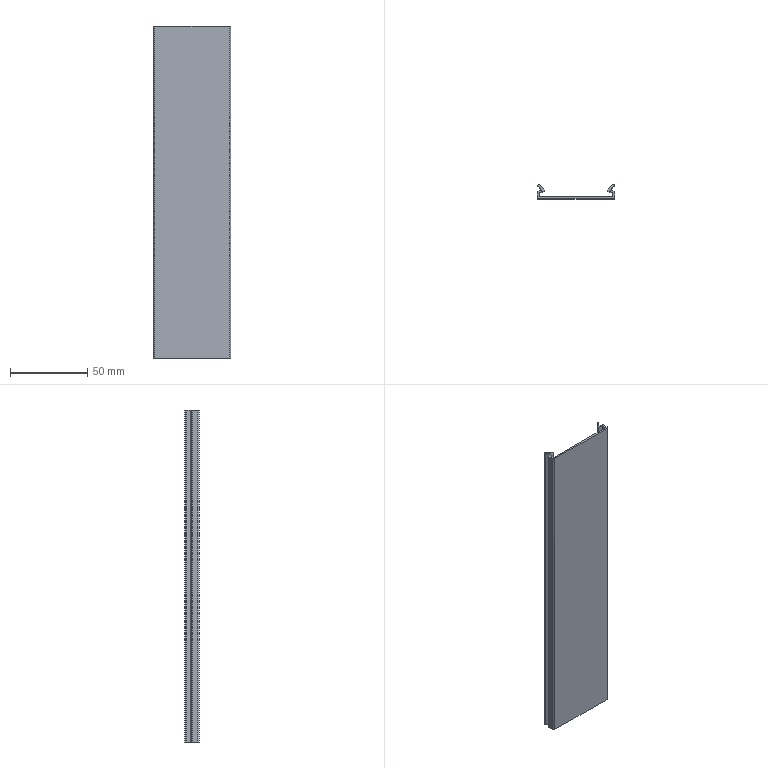Part | STEP file | 31E-01001CC12 | 1 solid | 32 faces | box 50 x 9.195 x 215 mm | volume 18858 mm3 | cylinder 16 | plane 16 | commonest cylinder face diameters 1 x8 1.2 x6 2 x2
STEP:
#1=CARTESIAN_POINT('',(0.2485,8.595,107.5));
#2=VERTEX_POINT('',#1);
#3=CARTESIAN_POINT('',(0.4243,8.171,107.5));
#4=VERTEX_POINT('',#3);
#5=CARTESIAN_POINT('',(0.8485,8.595,107.5));
#6=DIRECTION('',(0.,0.,-1.));
#7=AXIS2_PLACEMENT_3D('',#5,#6,$);
#8=CIRCLE('',#7,0.6);
#9=EDGE_CURVE('',#2,#4,#8,.F.);
#10=ORIENTED_EDGE('',*,*,#9,.F.);
#11=CARTESIAN_POINT('',(0.2485,8.595,-107.5));
#12=VERTEX_POINT('',#11);
#13=CARTESIAN_POINT('',(0.2485,8.595,107.5));
#14=DIRECTION('',(0.,0.,-1.));
#15=VECTOR('',#14,1.);
#16=LINE('',#13,#15);
#17=EDGE_CURVE('',#2,#12,#16,.T.);
#18=ORIENTED_EDGE('',*,*,#17,.T.);
#19=CARTESIAN_POINT('',(0.4243,8.171,-107.5));
#20=VERTEX_POINT('',#19);
#21=CARTESIAN_POINT('',(0.8485,8.595,-107.5));
#22=DIRECTION('',(0.,0.,-1.));
#23=AXIS2_PLACEMENT_3D('',#21,#22,$);
#24=CIRCLE('',#23,0.6);
#25=EDGE_CURVE('',#20,#12,#24,.T.);
#26=ORIENTED_EDGE('',*,*,#25,.F.);
#27=CARTESIAN_POINT('',(0.4243,8.171,107.5));
#28=DIRECTION('',(0.,0.,-1.));
#29=VECTOR('',#28,1.);
#30=LINE('',#27,#29);
#31=EDGE_CURVE('',#4,#20,#30,.T.);
#32=ORIENTED_EDGE('',*,*,#31,.F.);
#33=EDGE_LOOP('',(#10,#18,#26,#32));
#34=FACE_OUTER_BOUND('',#33,.T.);
#35=CARTESIAN_POINT('',(0.8485,8.595,107.5));
#36=DIRECTION('',(0.,0.,-1.));
#37=DIRECTION('',(1.,0.,0.));
#38=AXIS2_PLACEMENT_3D('',#35,#36,#37);
#39=CYLINDRICAL_SURFACE('',#38,0.6);
#40=ADVANCED_FACE('',(#34),#39,.T.);
#41=CARTESIAN_POINT('',(1.273,9.019,107.5));
#42=VERTEX_POINT('',#41);
#43=CARTESIAN_POINT('',(0.4243,9.019,107.5));
#44=VERTEX_POINT('',#43);
#45=CARTESIAN_POINT('',(1.273,9.019,107.5));
#46=CARTESIAN_POINT('',(1.219,9.073,107.5));
#47=CARTESIAN_POINT('',(1.158,9.118,107.5));
#48=CARTESIAN_POINT('',(1.089,9.152,107.5));
#49=CARTESIAN_POINT('',(0.9442,9.199,107.5));
#50=CARTESIAN_POINT('',(0.7916,9.2,107.5));
#51=CARTESIAN_POINT('',(0.7159,9.188,107.5));
#52=CARTESIAN_POINT('',(0.6071,9.152,107.5));
#53=CARTESIAN_POINT('',(0.5104,9.093,107.5));
#54=CARTESIAN_POINT('',(0.4796,9.07,107.5));
#55=CARTESIAN_POINT('',(0.4509,9.046,107.5));
#56=CARTESIAN_POINT('',(0.4243,9.019,107.5));
#57=B_SPLINE_CURVE_WITH_KNOTS('',5,(#45,#46,#47,#48,#49,#50,#51,#52,#53,#54,#55,#56),.UNSPECIFIED.,.F.,.U.,(6,3,3,6),(0.,0.5331,1.066,1.332),.UNSPECIFIED.);
#58=EDGE_CURVE('',#42,#44,#57,.T.);
#59=ORIENTED_EDGE('',*,*,#58,.T.);
#60=CARTESIAN_POINT('',(0.4243,9.019,107.5));
#61=CARTESIAN_POINT('',(0.3843,8.979,107.5));
#62=CARTESIAN_POINT('',(0.349,8.935,107.5));
#63=CARTESIAN_POINT('',(0.3192,8.886,107.5));
#64=CARTESIAN_POINT('',(0.2795,8.8,107.5));
#65=CARTESIAN_POINT('',(0.2574,8.708,107.5));
#66=CARTESIAN_POINT('',(0.2515,8.67,107.5));
#67=CARTESIAN_POINT('',(0.2485,8.633,107.5));
#68=CARTESIAN_POINT('',(0.2485,8.595,107.5));
#69=B_SPLINE_CURVE_WITH_KNOTS('',5,(#60,#61,#62,#63,#64,#65,#66,#67,#68),.UNSPECIFIED.,.F.,.U.,(6,3,6),(0.,0.3999,0.6659),.UNSPECIFIED.);
#70=EDGE_CURVE('',#44,#2,#69,.T.);
#71=ORIENTED_EDGE('',*,*,#70,.T.);
#72=ORIENTED_EDGE('',*,*,#9,.T.);
#73=CARTESIAN_POINT('',(2.898,5.697,107.5));
#74=VERTEX_POINT('',#73);
#75=CARTESIAN_POINT('',(1.661,6.934,107.5));
#76=DIRECTION('',(0.7071,-0.7071,0.));
#77=VECTOR('',#76,1.);
#78=LINE('',#75,#77);
#79=EDGE_CURVE('',#4,#74,#78,.T.);
#80=ORIENTED_EDGE('',*,*,#79,.T.);
#81=CARTESIAN_POINT('',(0.3706,5.02,107.5));
#82=VERTEX_POINT('',#81);
#83=CARTESIAN_POINT('',(1.634,5.359,107.5));
#84=DIRECTION('',(-0.9659,-0.2588,0.));
#85=VECTOR('',#84,1.);
#86=LINE('',#83,#85);
#87=EDGE_CURVE('',#74,#82,#86,.T.);
#88=ORIENTED_EDGE('',*,*,#87,.T.);
#89=CARTESIAN_POINT('',(0.,4.537,107.5));
#90=VERTEX_POINT('',#89);
#91=CARTESIAN_POINT('',(0.3706,5.02,107.5));
#92=CARTESIAN_POINT('',(0.32,5.007,107.5));
#93=CARTESIAN_POINT('',(0.2712,4.986,107.5));
#94=CARTESIAN_POINT('',(0.2253,4.96,107.5));
#95=CARTESIAN_POINT('',(0.1416,4.896,107.5));
#96=CARTESIAN_POINT('',(0.07725,4.812,107.5));
#97=CARTESIAN_POINT('',(0.05076,4.766,107.5));
#98=CARTESIAN_POINT('',(0.02052,4.693,107.5));
#99=CARTESIAN_POINT('',(0.005155,4.616,107.5));
#100=CARTESIAN_POINT('',(0.001709,4.589,107.5));
#101=CARTESIAN_POINT('',(0.,4.563,107.5));
#102=CARTESIAN_POINT('',(0.,4.537,107.5));
#103=B_SPLINE_CURVE_WITH_KNOTS('',5,(#91,#92,#93,#94,#95,#96,#97,#98,#99,#100,#101,#102),.UNSPECIFIED.,.F.,.U.,(6,3,3,6),(0.,0.3702,0.7405,0.9253),.UNSPECIFIED.);
#104=EDGE_CURVE('',#82,#90,#103,.T.);
#105=ORIENTED_EDGE('',*,*,#104,.T.);
#106=CARTESIAN_POINT('',(0.,1.,107.5));
#107=VERTEX_POINT('',#106);
#108=CARTESIAN_POINT('',(0.,2.769,107.5));
#109=DIRECTION('',(0.,-1.,0.));
#110=VECTOR('',#109,1.);
#111=LINE('',#108,#110);
#112=EDGE_CURVE('',#90,#107,#111,.T.);
#113=ORIENTED_EDGE('',*,*,#112,.T.);
#114=CARTESIAN_POINT('',(1.,0.,107.5));
#115=VERTEX_POINT('',#114);
#116=CARTESIAN_POINT('',(0.,1.,107.5));
#117=CARTESIAN_POINT('',(0.,0.902,107.5));
#118=CARTESIAN_POINT('',(0.012,0.804,107.5));
#119=CARTESIAN_POINT('',(0.036,0.708,107.5));
#120=CARTESIAN_POINT('',(0.107,0.5238,107.5));
#121=CARTESIAN_POINT('',(0.2204,0.3622,107.5));
#122=CARTESIAN_POINT('',(0.2868,0.2888,107.5));
#123=CARTESIAN_POINT('',(0.4361,0.1597,107.5));
#124=CARTESIAN_POINT('',(0.6122,0.0704,107.5));
#125=CARTESIAN_POINT('',(0.7053,0.03682,107.5));
#126=CARTESIAN_POINT('',(0.8215,0.01049,107.5));
#127=CARTESIAN_POINT('',(0.9393,0.001534,107.5));
#128=CARTESIAN_POINT('',(0.9596,0.0005109,107.5));
#129=CARTESIAN_POINT('',(0.9798,0.000000001,107.5));
#130=CARTESIAN_POINT('',(1.,0.000000001,107.5));
#131=B_SPLINE_CURVE_WITH_KNOTS('',5,(#116,#117,#118,#119,#120,#121,#122,#123,#124,#125,#126,#127,#128,#129,#130),.UNSPECIFIED.,.F.,.U.,(6,3,3,3,6),(0.,0.6928,1.386,2.078,2.221),.UNSPECIFIED.);
#132=EDGE_CURVE('',#107,#115,#131,.T.);
#133=ORIENTED_EDGE('',*,*,#132,.T.);
#134=CARTESIAN_POINT('',(49.,0.,107.5));
#135=VERTEX_POINT('',#134);
#136=CARTESIAN_POINT('',(25.,0.000000001,107.5));
#137=DIRECTION('',(1.,0.,0.));
#138=VECTOR('',#137,1.);
#139=LINE('',#136,#138);
#140=EDGE_CURVE('',#115,#135,#139,.T.);
#141=ORIENTED_EDGE('',*,*,#140,.T.);
#142=CARTESIAN_POINT('',(50.,1.,107.5));
#143=VERTEX_POINT('',#142);
#144=CARTESIAN_POINT('',(49.,0.000000001,107.5));
#145=CARTESIAN_POINT('',(49.098,0.000000001,107.5));
#146=CARTESIAN_POINT('',(49.196,0.012,107.5));
#147=CARTESIAN_POINT('',(49.292,0.036,107.5));
#148=CARTESIAN_POINT('',(49.476,0.107,107.5));
#149=CARTESIAN_POINT('',(49.638,0.2204,107.5));
#150=CARTESIAN_POINT('',(49.711,0.2868,107.5));
#151=CARTESIAN_POINT('',(49.84,0.4361,107.5));
#152=CARTESIAN_POINT('',(49.93,0.6122,107.5));
#153=CARTESIAN_POINT('',(49.963,0.7053,107.5));
#154=CARTESIAN_POINT('',(49.99,0.8215,107.5));
#155=CARTESIAN_POINT('',(49.998,0.9393,107.5));
#156=CARTESIAN_POINT('',(49.999,0.9596,107.5));
#157=CARTESIAN_POINT('',(50.,0.9798,107.5));
#158=CARTESIAN_POINT('',(50.,1.,107.5));
#159=B_SPLINE_CURVE_WITH_KNOTS('',5,(#144,#145,#146,#147,#148,#149,#150,#151,#152,#153,#154,#155,#156,#157,#158),.UNSPECIFIED.,.F.,.U.,(6,3,3,3,6),(0.,0.6928,1.386,2.078,2.221),.UNSPECIFIED.);
#160=EDGE_CURVE('',#135,#143,#159,.T.);
#161=ORIENTED_EDGE('',*,*,#160,.T.);
#162=CARTESIAN_POINT('',(50.,4.537,107.5));
#163=VERTEX_POINT('',#162);
#164=CARTESIAN_POINT('',(50.,2.769,107.5));
#165=DIRECTION('',(0.,1.,0.));
#166=VECTOR('',#165,1.);
#167=LINE('',#164,#166);
#168=EDGE_CURVE('',#143,#163,#167,.T.);
#169=ORIENTED_EDGE('',*,*,#168,.T.);
#170=CARTESIAN_POINT('',(49.629,5.02,107.5));
#171=VERTEX_POINT('',#170);
#172=CARTESIAN_POINT('',(50.,4.537,107.5));
#173=CARTESIAN_POINT('',(50.,4.589,107.5));
#174=CARTESIAN_POINT('',(49.993,4.642,107.5));
#175=CARTESIAN_POINT('',(49.979,4.693,107.5));
#176=CARTESIAN_POINT('',(49.939,4.791,107.5));
#177=CARTESIAN_POINT('',(49.875,4.874,107.5));
#178=CARTESIAN_POINT('',(49.837,4.912,107.5));
#179=CARTESIAN_POINT('',(49.774,4.96,107.5));
#180=CARTESIAN_POINT('',(49.704,4.995,107.5));
#181=CARTESIAN_POINT('',(49.679,5.005,107.5));
#182=CARTESIAN_POINT('',(49.655,5.013,107.5));
#183=CARTESIAN_POINT('',(49.629,5.02,107.5));
#184=B_SPLINE_CURVE_WITH_KNOTS('',5,(#172,#173,#174,#175,#176,#177,#178,#179,#180,#181,#182,#183),.UNSPECIFIED.,.F.,.U.,(6,3,3,6),(0.,0.3702,0.7405,0.9253),.UNSPECIFIED.);
#185=EDGE_CURVE('',#163,#171,#184,.T.);
#186=ORIENTED_EDGE('',*,*,#185,.T.);
#187=CARTESIAN_POINT('',(47.102,5.697,107.5));
#188=VERTEX_POINT('',#187);
#189=CARTESIAN_POINT('',(48.366,5.359,107.5));
#190=DIRECTION('',(-0.9659,0.2588,0.));
#191=VECTOR('',#190,1.);
#192=LINE('',#189,#191);
#193=EDGE_CURVE('',#171,#188,#192,.T.);
#194=ORIENTED_EDGE('',*,*,#193,.T.);
#195=CARTESIAN_POINT('',(49.576,8.171,107.5));
#196=VERTEX_POINT('',#195);
#197=CARTESIAN_POINT('',(48.339,6.934,107.5));
#198=DIRECTION('',(0.7071,0.7071,0.));
#199=VECTOR('',#198,1.);
#200=LINE('',#197,#199);
#201=EDGE_CURVE('',#188,#196,#200,.T.);
#202=ORIENTED_EDGE('',*,*,#201,.T.);
#203=CARTESIAN_POINT('',(49.751,8.595,107.5));
#204=VERTEX_POINT('',#203);
#205=CARTESIAN_POINT('',(49.576,8.171,107.5));
#206=CARTESIAN_POINT('',(49.629,8.224,107.5));
#207=CARTESIAN_POINT('',(49.674,8.286,107.5));
#208=CARTESIAN_POINT('',(49.709,8.354,107.5));
#209=CARTESIAN_POINT('',(49.738,8.445,107.5));
#210=CARTESIAN_POINT('',(49.749,8.539,107.5));
#211=CARTESIAN_POINT('',(49.751,8.557,107.5));
#212=CARTESIAN_POINT('',(49.751,8.576,107.5));
#213=CARTESIAN_POINT('',(49.751,8.595,107.5));
#214=B_SPLINE_CURVE_WITH_KNOTS('',5,(#205,#206,#207,#208,#209,#210,#211,#212,#213),.UNSPECIFIED.,.F.,.U.,(6,3,6),(0.,0.5331,0.6664),.UNSPECIFIED.);
#215=EDGE_CURVE('',#196,#204,#214,.T.);
#216=ORIENTED_EDGE('',*,*,#215,.T.);
#217=CARTESIAN_POINT('',(49.576,9.019,107.5));
#218=VERTEX_POINT('',#217);
#219=CARTESIAN_POINT('',(49.751,8.595,107.5));
#220=CARTESIAN_POINT('',(49.751,8.652,107.5));
#221=CARTESIAN_POINT('',(49.745,8.708,107.5));
#222=CARTESIAN_POINT('',(49.731,8.764,107.5));
#223=CARTESIAN_POINT('',(49.699,8.853,107.5));
#224=CARTESIAN_POINT('',(49.649,8.933,107.5));
#225=CARTESIAN_POINT('',(49.627,8.964,107.5));
#226=CARTESIAN_POINT('',(49.602,8.993,107.5));
#227=CARTESIAN_POINT('',(49.576,9.019,107.5));
#228=B_SPLINE_CURVE_WITH_KNOTS('',5,(#219,#220,#221,#222,#223,#224,#225,#226,#227),.UNSPECIFIED.,.F.,.U.,(6,3,6),(0.6664,1.066,1.332),.UNSPECIFIED.);
#229=EDGE_CURVE('',#204,#218,#228,.T.);
#230=ORIENTED_EDGE('',*,*,#229,.T.);
#231=CARTESIAN_POINT('',(48.727,9.019,107.5));
#232=VERTEX_POINT('',#231);
#233=CARTESIAN_POINT('',(49.576,9.019,107.5));
#234=CARTESIAN_POINT('',(49.522,9.073,107.5));
#235=CARTESIAN_POINT('',(49.461,9.118,107.5));
#236=CARTESIAN_POINT('',(49.392,9.152,107.5));
#237=CARTESIAN_POINT('',(49.247,9.199,107.5));
#238=CARTESIAN_POINT('',(49.095,9.2,107.5));
#239=CARTESIAN_POINT('',(49.019,9.188,107.5));
#240=CARTESIAN_POINT('',(48.91,9.152,107.5));
#241=CARTESIAN_POINT('',(48.813,9.093,107.5));
#242=CARTESIAN_POINT('',(48.782,9.07,107.5));
#243=CARTESIAN_POINT('',(48.754,9.046,107.5));
#244=CARTESIAN_POINT('',(48.727,9.019,107.5));
#245=B_SPLINE_CURVE_WITH_KNOTS('',5,(#233,#234,#235,#236,#237,#238,#239,#240,#241,#242,#243,#244),.UNSPECIFIED.,.F.,.U.,(6,3,3,6),(0.,0.5331,1.066,1.332),.UNSPECIFIED.);
#246=EDGE_CURVE('',#218,#232,#245,.T.);
#247=ORIENTED_EDGE('',*,*,#246,.T.);
#248=CARTESIAN_POINT('',(45.396,5.688,107.5));
#249=VERTEX_POINT('',#248);
#250=CARTESIAN_POINT('',(47.062,7.354,107.5));
#251=DIRECTION('',(-0.7071,-0.7071,0.));
#252=VECTOR('',#251,1.);
#253=LINE('',#250,#252);
#254=EDGE_CURVE('',#232,#249,#253,.T.);
#255=ORIENTED_EDGE('',*,*,#254,.T.);
#256=CARTESIAN_POINT('',(45.25,5.335,107.5));
#257=VERTEX_POINT('',#256);
#258=CARTESIAN_POINT('',(45.396,5.688,107.5));
#259=CARTESIAN_POINT('',(45.363,5.655,107.5));
#260=CARTESIAN_POINT('',(45.334,5.618,107.5));
#261=CARTESIAN_POINT('',(45.309,5.577,107.5));
#262=CARTESIAN_POINT('',(45.276,5.506,107.5));
#263=CARTESIAN_POINT('',(45.257,5.429,107.5));
#264=CARTESIAN_POINT('',(45.252,5.398,107.5));
#265=CARTESIAN_POINT('',(45.25,5.366,107.5));
#266=CARTESIAN_POINT('',(45.25,5.335,107.5));
#267=B_SPLINE_CURVE_WITH_KNOTS('',5,(#258,#259,#260,#261,#262,#263,#264,#265,#266),.UNSPECIFIED.,.F.,.U.,(6,3,6),(0.,0.3332,0.5549),.UNSPECIFIED.);
#268=EDGE_CURVE('',#249,#257,#267,.T.);
#269=ORIENTED_EDGE('',*,*,#268,.T.);
#270=CARTESIAN_POINT('',(45.621,4.852,107.5));
#271=VERTEX_POINT('',#270);
#272=CARTESIAN_POINT('',(45.25,5.335,107.5));
#273=CARTESIAN_POINT('',(45.25,5.283,107.5));
#274=CARTESIAN_POINT('',(45.257,5.23,107.5));
#275=CARTESIAN_POINT('',(45.27,5.179,107.5));
#276=CARTESIAN_POINT('',(45.311,5.081,107.5));
#277=CARTESIAN_POINT('',(45.375,4.998,107.5));
#278=CARTESIAN_POINT('',(45.413,4.96,107.5));
#279=CARTESIAN_POINT('',(45.476,4.912,107.5));
#280=CARTESIAN_POINT('',(45.546,4.877,107.5));
#281=CARTESIAN_POINT('',(45.57,4.867,107.5));
#282=CARTESIAN_POINT('',(45.595,4.859,107.5));
#283=CARTESIAN_POINT('',(45.621,4.852,107.5));
#284=B_SPLINE_CURVE_WITH_KNOTS('',5,(#272,#273,#274,#275,#276,#277,#278,#279,#280,#281,#282,#283),.UNSPECIFIED.,.F.,.U.,(6,3,3,6),(0.,0.3702,0.7405,0.9253),.UNSPECIFIED.);
#285=EDGE_CURVE('',#257,#271,#284,.T.);
#286=ORIENTED_EDGE('',*,*,#285,.T.);
#287=CARTESIAN_POINT('',(48.8,4.,107.5));
#288=VERTEX_POINT('',#287);
#289=CARTESIAN_POINT('',(47.21,4.426,107.5));
#290=DIRECTION('',(0.9659,-0.2588,0.));
#291=VECTOR('',#290,1.);
#292=LINE('',#289,#291);
#293=EDGE_CURVE('',#271,#288,#292,.T.);
#294=ORIENTED_EDGE('',*,*,#293,.T.);
#295=CARTESIAN_POINT('',(48.8,1.7,107.5));
#296=VERTEX_POINT('',#295);
#297=CARTESIAN_POINT('',(48.8,2.85,107.5));
#298=DIRECTION('',(0.,-1.,0.));
#299=VECTOR('',#298,1.);
#300=LINE('',#297,#299);
#301=EDGE_CURVE('',#288,#296,#300,.T.);
#302=ORIENTED_EDGE('',*,*,#301,.T.);
#303=CARTESIAN_POINT('',(48.3,1.2,107.5));
#304=VERTEX_POINT('',#303);
#305=CARTESIAN_POINT('',(48.3,1.7,107.5));
#306=DIRECTION('',(0.,0.,-1.));
#307=AXIS2_PLACEMENT_3D('',#305,#306,$);
#308=CIRCLE('',#307,0.5);
#309=EDGE_CURVE('',#296,#304,#308,.T.);
#310=ORIENTED_EDGE('',*,*,#309,.T.);
#311=CARTESIAN_POINT('',(1.7,1.2,107.5));
#312=VERTEX_POINT('',#311);
#313=CARTESIAN_POINT('',(25.,1.2,107.5));
#314=DIRECTION('',(-1.,0.,0.));
#315=VECTOR('',#314,1.);
#316=LINE('',#313,#315);
#317=EDGE_CURVE('',#304,#312,#316,.T.);
#318=ORIENTED_EDGE('',*,*,#317,.T.);
#319=CARTESIAN_POINT('',(1.2,1.7,107.5));
#320=VERTEX_POINT('',#319);
#321=CARTESIAN_POINT('',(1.7,1.7,107.5));
#322=DIRECTION('',(0.,0.,-1.));
#323=AXIS2_PLACEMENT_3D('',#321,#322,$);
#324=CIRCLE('',#323,0.5);
#325=EDGE_CURVE('',#312,#320,#324,.T.);
#326=ORIENTED_EDGE('',*,*,#325,.T.);
#327=CARTESIAN_POINT('',(1.2,4.,107.5));
#328=VERTEX_POINT('',#327);
#329=CARTESIAN_POINT('',(1.2,2.85,107.5));
#330=DIRECTION('',(0.,1.,0.));
#331=VECTOR('',#330,1.);
#332=LINE('',#329,#331);
#333=EDGE_CURVE('',#320,#328,#332,.T.);
#334=ORIENTED_EDGE('',*,*,#333,.T.);
#335=CARTESIAN_POINT('',(4.379,4.852,107.5));
#336=VERTEX_POINT('',#335);
#337=CARTESIAN_POINT('',(2.79,4.426,107.5));
#338=DIRECTION('',(0.9659,0.2588,0.));
#339=VECTOR('',#338,1.);
#340=LINE('',#337,#339);
#341=EDGE_CURVE('',#328,#336,#340,.T.);
#342=ORIENTED_EDGE('',*,*,#341,.T.);
#343=CARTESIAN_POINT('',(4.75,5.335,107.5));
#344=VERTEX_POINT('',#343);
#345=CARTESIAN_POINT('',(4.379,4.852,107.5));
#346=CARTESIAN_POINT('',(4.446,4.87,107.5));
#347=CARTESIAN_POINT('',(4.51,4.899,107.5));
#348=CARTESIAN_POINT('',(4.568,4.94,107.5));
#349=CARTESIAN_POINT('',(4.662,5.034,107.5));
#350=CARTESIAN_POINT('',(4.722,5.152,107.5));
#351=CARTESIAN_POINT('',(4.741,5.212,107.5));
#352=CARTESIAN_POINT('',(4.75,5.273,107.5));
#353=CARTESIAN_POINT('',(4.75,5.335,107.5));
#354=B_SPLINE_CURVE_WITH_KNOTS('',5,(#345,#346,#347,#348,#349,#350,#351,#352,#353),.UNSPECIFIED.,.F.,.U.,(6,3,6),(0.,0.4899,0.9256),.UNSPECIFIED.);
#355=EDGE_CURVE('',#336,#344,#354,.T.);
#356=ORIENTED_EDGE('',*,*,#355,.T.);
#357=CARTESIAN_POINT('',(4.604,5.688,107.5));
#358=VERTEX_POINT('',#357);
#359=CARTESIAN_POINT('',(4.75,5.335,107.5));
#360=CARTESIAN_POINT('',(4.75,5.343,107.5));
#361=CARTESIAN_POINT('',(4.75,5.35,107.5));
#362=CARTESIAN_POINT('',(4.75,5.358,107.5));
#363=CARTESIAN_POINT('',(4.745,5.435,107.5));
#364=CARTESIAN_POINT('',(4.726,5.51,107.5));
#365=CARTESIAN_POINT('',(4.697,5.575,107.5));
#366=CARTESIAN_POINT('',(4.657,5.634,107.5));
#367=CARTESIAN_POINT('',(4.607,5.685,107.5));
#368=CARTESIAN_POINT('',(4.606,5.686,107.5));
#369=CARTESIAN_POINT('',(4.605,5.687,107.5));
#370=CARTESIAN_POINT('',(4.604,5.688,107.5));
#371=B_SPLINE_CURVE_WITH_KNOTS('',5,(#359,#360,#361,#362,#363,#364,#365,#366,#367,#368,#369,#370),.UNSPECIFIED.,.F.,.U.,(6,3,3,6),(0.9256,0.9798,1.47,1.481),.UNSPECIFIED.);
#372=EDGE_CURVE('',#344,#358,#371,.T.);
#373=ORIENTED_EDGE('',*,*,#372,.T.);
#374=CARTESIAN_POINT('',(2.938,7.354,107.5));
#375=DIRECTION('',(-0.7071,0.7071,0.));
#376=VECTOR('',#375,1.);
#377=LINE('',#374,#376);
#378=EDGE_CURVE('',#358,#42,#377,.T.);
#379=ORIENTED_EDGE('',*,*,#378,.T.);
#380=EDGE_LOOP('',(#59,#71,#72,#80,#88,#105,#113,#133,#141,#161,#169,#186,#194,#202,#216,#230,#247,#255,#269,#286,#294,#302,#310,#318,#326,#334,#342,#356,#373,#379));
#381=FACE_OUTER_BOUND('',#380,.T.);
#382=CARTESIAN_POINT('',(0.,1.2,107.5));
#383=DIRECTION('',(0.,0.,-1.));
#384=DIRECTION('',(-1.,0.,0.));
#385=AXIS2_PLACEMENT_3D('',#382,#383,#384);
#386=PLANE('',#385);
#387=ADVANCED_FACE('',(#381),#386,.F.);
#388=ORIENTED_EDGE('',*,*,#17,.F.);
#389=ORIENTED_EDGE('',*,*,#70,.F.);
#390=CARTESIAN_POINT('',(0.4243,9.019,-107.5));
#391=VERTEX_POINT('',#390);
#392=CARTESIAN_POINT('',(0.4243,9.019,107.5));
#393=DIRECTION('',(0.,0.,-1.));
#394=VECTOR('',#393,1.);
#395=LINE('',#392,#394);
#396=EDGE_CURVE('',#44,#391,#395,.T.);
#397=ORIENTED_EDGE('',*,*,#396,.T.);
#398=CARTESIAN_POINT('',(0.8485,8.595,-107.5));
#399=DIRECTION('',(0.,0.,-1.));
#400=AXIS2_PLACEMENT_3D('',#398,#399,$);
#401=CIRCLE('',#400,0.6);
#402=EDGE_CURVE('',#12,#391,#401,.T.);
#403=ORIENTED_EDGE('',*,*,#402,.F.);
#404=EDGE_LOOP('',(#388,#389,#397,#403));
#405=FACE_OUTER_BOUND('',#404,.T.);
#406=CARTESIAN_POINT('',(0.8485,8.595,107.5));
#407=DIRECTION('',(0.,0.,-1.));
#408=DIRECTION('',(-1.,0.,0.));
#409=AXIS2_PLACEMENT_3D('',#406,#407,#408);
#410=CYLINDRICAL_SURFACE('',#409,0.6);
#411=ADVANCED_FACE('',(#405),#410,.T.);
#412=CARTESIAN_POINT('',(2.898,5.697,-107.5));
#413=VERTEX_POINT('',#412);
#414=CARTESIAN_POINT('',(1.661,6.934,-107.5));
#415=DIRECTION('',(0.7071,-0.7071,0.));
#416=VECTOR('',#415,1.);
#417=LINE('',#414,#416);
#418=EDGE_CURVE('',#20,#413,#417,.T.);
#419=ORIENTED_EDGE('',*,*,#418,.F.);
#420=ORIENTED_EDGE('',*,*,#25,.T.);
#421=ORIENTED_EDGE('',*,*,#402,.T.);
#422=CARTESIAN_POINT('',(1.273,9.019,-107.5));
#423=VERTEX_POINT('',#422);
#424=CARTESIAN_POINT('',(0.8485,8.595,-107.5));
#425=DIRECTION('',(0.,0.,-1.));
#426=AXIS2_PLACEMENT_3D('',#424,#425,$);
#427=CIRCLE('',#426,0.6);
#428=EDGE_CURVE('',#391,#423,#427,.T.);
#429=ORIENTED_EDGE('',*,*,#428,.T.);
#430=CARTESIAN_POINT('',(4.604,5.688,-107.5));
#431=VERTEX_POINT('',#430);
#432=CARTESIAN_POINT('',(2.938,7.354,-107.5));
#433=DIRECTION('',(-0.7071,0.7071,0.));
#434=VECTOR('',#433,1.);
#435=LINE('',#432,#434);
#436=EDGE_CURVE('',#431,#423,#435,.T.);
#437=ORIENTED_EDGE('',*,*,#436,.F.);
#438=CARTESIAN_POINT('',(4.75,5.335,-107.5));
#439=VERTEX_POINT('',#438);
#440=CARTESIAN_POINT('',(4.25,5.335,-107.5));
#441=DIRECTION('',(0.,0.,-1.));
#442=AXIS2_PLACEMENT_3D('',#440,#441,$);
#443=CIRCLE('',#442,0.5);
#444=EDGE_CURVE('',#431,#439,#443,.T.);
#445=ORIENTED_EDGE('',*,*,#444,.T.);
#446=CARTESIAN_POINT('',(4.379,4.852,-107.5));
#447=VERTEX_POINT('',#446);
#448=CARTESIAN_POINT('',(4.25,5.335,-107.5));
#449=DIRECTION('',(0.,0.,-1.));
#450=AXIS2_PLACEMENT_3D('',#448,#449,$);
#451=CIRCLE('',#450,0.5);
#452=EDGE_CURVE('',#439,#447,#451,.T.);
#453=ORIENTED_EDGE('',*,*,#452,.T.);
#454=CARTESIAN_POINT('',(1.2,4.,-107.5));
#455=VERTEX_POINT('',#454);
#456=CARTESIAN_POINT('',(2.79,4.426,-107.5));
#457=DIRECTION('',(0.9659,0.2588,0.));
#458=VECTOR('',#457,1.);
#459=LINE('',#456,#458);
#460=EDGE_CURVE('',#455,#447,#459,.T.);
#461=ORIENTED_EDGE('',*,*,#460,.F.);
#462=CARTESIAN_POINT('',(1.2,1.7,-107.5));
#463=VERTEX_POINT('',#462);
#464=CARTESIAN_POINT('',(1.2,2.85,-107.5));
#465=DIRECTION('',(0.,1.,0.));
#466=VECTOR('',#465,1.);
#467=LINE('',#464,#466);
#468=EDGE_CURVE('',#463,#455,#467,.T.);
#469=ORIENTED_EDGE('',*,*,#468,.F.);
#470=CARTESIAN_POINT('',(1.7,1.2,-107.5));
#471=VERTEX_POINT('',#470);
#472=CARTESIAN_POINT('',(1.2,1.7,-107.5));
#473=CARTESIAN_POINT('',(1.2,1.637,-107.5));
#474=CARTESIAN_POINT('',(1.21,1.574,-107.5));
#475=CARTESIAN_POINT('',(1.23,1.514,-107.5));
#476=CARTESIAN_POINT('',(1.288,1.4,-107.5));
#477=CARTESIAN_POINT('',(1.377,1.31,-107.5));
#478=CARTESIAN_POINT('',(1.429,1.273,-107.5));
#479=CARTESIAN_POINT('',(1.514,1.23,-107.5));
#480=CARTESIAN_POINT('',(1.606,1.207,-107.5));
#481=CARTESIAN_POINT('',(1.637,1.202,-107.5));
#482=CARTESIAN_POINT('',(1.669,1.2,-107.5));
#483=CARTESIAN_POINT('',(1.7,1.2,-107.5));
#484=B_SPLINE_CURVE_WITH_KNOTS('',5,(#472,#473,#474,#475,#476,#477,#478,#479,#480,#481,#482,#483),.UNSPECIFIED.,.F.,.U.,(6,3,3,6),(0.,0.4443,0.8886,1.11),.UNSPECIFIED.);
#485=EDGE_CURVE('',#463,#471,#484,.T.);
#486=ORIENTED_EDGE('',*,*,#485,.T.);
#487=CARTESIAN_POINT('',(48.3,1.2,-107.5));
#488=VERTEX_POINT('',#487);
#489=CARTESIAN_POINT('',(25.,1.2,-107.5));
#490=DIRECTION('',(-1.,0.,0.));
#491=VECTOR('',#490,1.);
#492=LINE('',#489,#491);
#493=EDGE_CURVE('',#488,#471,#492,.T.);
#494=ORIENTED_EDGE('',*,*,#493,.F.);
#495=CARTESIAN_POINT('',(48.8,1.7,-107.5));
#496=VERTEX_POINT('',#495);
#497=CARTESIAN_POINT('',(48.3,1.2,-107.5));
#498=CARTESIAN_POINT('',(48.363,1.2,-107.5));
#499=CARTESIAN_POINT('',(48.426,1.21,-107.5));
#500=CARTESIAN_POINT('',(48.486,1.23,-107.5));
#501=CARTESIAN_POINT('',(48.6,1.288,-107.5));
#502=CARTESIAN_POINT('',(48.69,1.377,-107.5));
#503=CARTESIAN_POINT('',(48.727,1.429,-107.5));
#504=CARTESIAN_POINT('',(48.77,1.514,-107.5));
#505=CARTESIAN_POINT('',(48.793,1.606,-107.5));
#506=CARTESIAN_POINT('',(48.798,1.637,-107.5));
#507=CARTESIAN_POINT('',(48.8,1.669,-107.5));
#508=CARTESIAN_POINT('',(48.8,1.7,-107.5));
#509=B_SPLINE_CURVE_WITH_KNOTS('',5,(#497,#498,#499,#500,#501,#502,#503,#504,#505,#506,#507,#508),.UNSPECIFIED.,.F.,.U.,(6,3,3,6),(0.,0.4443,0.8886,1.11),.UNSPECIFIED.);
#510=EDGE_CURVE('',#488,#496,#509,.T.);
#511=ORIENTED_EDGE('',*,*,#510,.T.);
#512=CARTESIAN_POINT('',(48.8,4.,-107.5));
#513=VERTEX_POINT('',#512);
#514=CARTESIAN_POINT('',(48.8,2.85,-107.5));
#515=DIRECTION('',(0.,-1.,0.));
#516=VECTOR('',#515,1.);
#517=LINE('',#514,#516);
#518=EDGE_CURVE('',#513,#496,#517,.T.);
#519=ORIENTED_EDGE('',*,*,#518,.F.);
#520=CARTESIAN_POINT('',(45.621,4.852,-107.5));
#521=VERTEX_POINT('',#520);
#522=CARTESIAN_POINT('',(47.21,4.426,-107.5));
#523=DIRECTION('',(0.9659,-0.2588,0.));
#524=VECTOR('',#523,1.);
#525=LINE('',#522,#524);
#526=EDGE_CURVE('',#521,#513,#525,.T.);
#527=ORIENTED_EDGE('',*,*,#526,.F.);
#528=CARTESIAN_POINT('',(45.25,5.335,-107.5));
#529=VERTEX_POINT('',#528);
#530=CARTESIAN_POINT('',(45.75,5.335,-107.5));
#531=DIRECTION('',(0.,0.,-1.));
#532=AXIS2_PLACEMENT_3D('',#530,#531,$);
#533=CIRCLE('',#532,0.5);
#534=EDGE_CURVE('',#521,#529,#533,.T.);
#535=ORIENTED_EDGE('',*,*,#534,.T.);
#536=CARTESIAN_POINT('',(45.396,5.688,-107.5));
#537=VERTEX_POINT('',#536);
#538=CARTESIAN_POINT('',(45.75,5.335,-107.5));
#539=DIRECTION('',(0.,0.,-1.));
#540=AXIS2_PLACEMENT_3D('',#538,#539,$);
#541=CIRCLE('',#540,0.5);
#542=EDGE_CURVE('',#529,#537,#541,.T.);
#543=ORIENTED_EDGE('',*,*,#542,.T.);
#544=CARTESIAN_POINT('',(48.727,9.019,-107.5));
#545=VERTEX_POINT('',#544);
#546=CARTESIAN_POINT('',(47.062,7.354,-107.5));
#547=DIRECTION('',(-0.7071,-0.7071,0.));
#548=VECTOR('',#547,1.);
#549=LINE('',#546,#548);
#550=EDGE_CURVE('',#545,#537,#549,.T.);
#551=ORIENTED_EDGE('',*,*,#550,.F.);
#552=CARTESIAN_POINT('',(49.576,9.019,-107.5));
#553=VERTEX_POINT('',#552);
#554=CARTESIAN_POINT('',(49.151,8.595,-107.5));
#555=DIRECTION('',(0.,0.,-1.));
#556=AXIS2_PLACEMENT_3D('',#554,#555,$);
#557=CIRCLE('',#556,0.6);
#558=EDGE_CURVE('',#545,#553,#557,.T.);
#559=ORIENTED_EDGE('',*,*,#558,.T.);
#560=CARTESIAN_POINT('',(49.751,8.595,-107.5));
#561=VERTEX_POINT('',#560);
#562=CARTESIAN_POINT('',(49.151,8.595,-107.5));
#563=DIRECTION('',(0.,0.,-1.));
#564=AXIS2_PLACEMENT_3D('',#562,#563,$);
#565=CIRCLE('',#564,0.6);
#566=EDGE_CURVE('',#553,#561,#565,.T.);
#567=ORIENTED_EDGE('',*,*,#566,.T.);
#568=CARTESIAN_POINT('',(49.576,8.171,-107.5));
#569=VERTEX_POINT('',#568);
#570=CARTESIAN_POINT('',(49.151,8.595,-107.5));
#571=DIRECTION('',(0.,0.,-1.));
#572=AXIS2_PLACEMENT_3D('',#570,#571,$);
#573=CIRCLE('',#572,0.6);
#574=EDGE_CURVE('',#561,#569,#573,.T.);
#575=ORIENTED_EDGE('',*,*,#574,.T.);
#576=CARTESIAN_POINT('',(47.102,5.697,-107.5));
#577=VERTEX_POINT('',#576);
#578=CARTESIAN_POINT('',(48.339,6.934,-107.5));
#579=DIRECTION('',(0.7071,0.7071,0.));
#580=VECTOR('',#579,1.);
#581=LINE('',#578,#580);
#582=EDGE_CURVE('',#577,#569,#581,.T.);
#583=ORIENTED_EDGE('',*,*,#582,.F.);
#584=CARTESIAN_POINT('',(49.629,5.02,-107.5));
#585=VERTEX_POINT('',#584);
#586=CARTESIAN_POINT('',(48.366,5.359,-107.5));
#587=DIRECTION('',(-0.9659,0.2588,0.));
#588=VECTOR('',#587,1.);
#589=LINE('',#586,#588);
#590=EDGE_CURVE('',#585,#577,#589,.T.);
#591=ORIENTED_EDGE('',*,*,#590,.F.);
#592=CARTESIAN_POINT('',(50.,4.537,-107.5));
#593=VERTEX_POINT('',#592);
#594=CARTESIAN_POINT('',(49.5,4.537,-107.5));
#595=DIRECTION('',(0.,0.,-1.));
#596=AXIS2_PLACEMENT_3D('',#594,#595,$);
#597=CIRCLE('',#596,0.5);
#598=EDGE_CURVE('',#585,#593,#597,.T.);
#599=ORIENTED_EDGE('',*,*,#598,.T.);
#600=CARTESIAN_POINT('',(50.,1.,-107.5));
#601=VERTEX_POINT('',#600);
#602=CARTESIAN_POINT('',(50.,2.769,-107.5));
#603=DIRECTION('',(0.,1.,0.));
#604=VECTOR('',#603,1.);
#605=LINE('',#602,#604);
#606=EDGE_CURVE('',#601,#593,#605,.T.);
#607=ORIENTED_EDGE('',*,*,#606,.F.);
#608=CARTESIAN_POINT('',(49.,0.,-107.5));
#609=VERTEX_POINT('',#608);
#610=CARTESIAN_POINT('',(49.,1.,-107.5));
#611=DIRECTION('',(0.,0.,-1.));
#612=AXIS2_PLACEMENT_3D('',#610,#611,$);
#613=CIRCLE('',#612,1.);
#614=EDGE_CURVE('',#601,#609,#613,.T.);
#615=ORIENTED_EDGE('',*,*,#614,.T.);
#616=CARTESIAN_POINT('',(1.,0.,-107.5));
#617=VERTEX_POINT('',#616);
#618=CARTESIAN_POINT('',(25.,0.000000001,-107.5));
#619=DIRECTION('',(1.,0.,0.));
#620=VECTOR('',#619,1.);
#621=LINE('',#618,#620);
#622=EDGE_CURVE('',#617,#609,#621,.T.);
#623=ORIENTED_EDGE('',*,*,#622,.F.);
#624=CARTESIAN_POINT('',(0.,1.,-107.5));
#625=VERTEX_POINT('',#624);
#626=CARTESIAN_POINT('',(1.,1.,-107.5));
#627=DIRECTION('',(0.,0.,-1.));
#628=AXIS2_PLACEMENT_3D('',#626,#627,$);
#629=CIRCLE('',#628,1.);
#630=EDGE_CURVE('',#617,#625,#629,.T.);
#631=ORIENTED_EDGE('',*,*,#630,.T.);
#632=CARTESIAN_POINT('',(0.,4.537,-107.5));
#633=VERTEX_POINT('',#632);
#634=CARTESIAN_POINT('',(0.,2.769,-107.5));
#635=DIRECTION('',(0.,-1.,0.));
#636=VECTOR('',#635,1.);
#637=LINE('',#634,#636);
#638=EDGE_CURVE('',#633,#625,#637,.T.);
#639=ORIENTED_EDGE('',*,*,#638,.F.);
#640=CARTESIAN_POINT('',(0.3706,5.02,-107.5));
#641=VERTEX_POINT('',#640);
#642=CARTESIAN_POINT('',(0.5,4.537,-107.5));
#643=DIRECTION('',(0.,0.,-1.));
#644=AXIS2_PLACEMENT_3D('',#642,#643,$);
#645=CIRCLE('',#644,0.5);
#646=EDGE_CURVE('',#633,#641,#645,.T.);
#647=ORIENTED_EDGE('',*,*,#646,.T.);
#648=CARTESIAN_POINT('',(1.634,5.359,-107.5));
#649=DIRECTION('',(-0.9659,-0.2588,0.));
#650=VECTOR('',#649,1.);
#651=LINE('',#648,#650);
#652=EDGE_CURVE('',#413,#641,#651,.T.);
#653=ORIENTED_EDGE('',*,*,#652,.F.);
#654=EDGE_LOOP('',(#419,#420,#421,#429,#437,#445,#453,#461,#469,#486,#494,#511,#519,#527,#535,#543,#551,#559,#567,#575,#583,#591,#599,#607,#615,#623,#631,#639,#647,#653));
#655=FACE_OUTER_BOUND('',#654,.T.);
#656=CARTESIAN_POINT('',(0.,1.2,-107.5));
#657=DIRECTION('',(0.,0.,-1.));
#658=DIRECTION('',(-1.,0.,0.));
#659=AXIS2_PLACEMENT_3D('',#656,#657,#658);
#660=PLANE('',#659);
#661=ADVANCED_FACE('',(#655),#660,.T.);
#662=ORIENTED_EDGE('',*,*,#79,.F.);
#663=ORIENTED_EDGE('',*,*,#31,.T.);
#664=ORIENTED_EDGE('',*,*,#418,.T.);
#665=CARTESIAN_POINT('',(2.898,5.697,0.));
#666=DIRECTION('',(0.,0.,-1.));
#667=VECTOR('',#666,1.);
#668=LINE('',#665,#667);
#669=EDGE_CURVE('',#74,#413,#668,.T.);
#670=ORIENTED_EDGE('',*,*,#669,.F.);
#671=EDGE_LOOP('',(#662,#663,#664,#670));
#672=FACE_OUTER_BOUND('',#671,.T.);
#673=CARTESIAN_POINT('',(2.898,5.697,107.5));
#674=DIRECTION('',(0.7071,0.7071,0.));
#675=DIRECTION('',(-0.7071,0.7071,0.));
#676=AXIS2_PLACEMENT_3D('',#673,#674,#675);
#677=PLANE('',#676);
#678=ADVANCED_FACE('',(#672),#677,.F.);
#679=ORIENTED_EDGE('',*,*,#396,.F.);
#680=ORIENTED_EDGE('',*,*,#58,.F.);
#681=CARTESIAN_POINT('',(1.273,9.019,107.5));
#682=DIRECTION('',(0.,0.,-1.));
#683=VECTOR('',#682,1.);
#684=LINE('',#681,#683);
#685=EDGE_CURVE('',#423,#42,#684,.F.);
#686=ORIENTED_EDGE('',*,*,#685,.F.);
#687=ORIENTED_EDGE('',*,*,#428,.F.);
#688=EDGE_LOOP('',(#679,#680,#686,#687));
#689=FACE_OUTER_BOUND('',#688,.T.);
#690=CARTESIAN_POINT('',(0.8485,8.595,107.5));
#691=DIRECTION('',(0.,0.,-1.));
#692=DIRECTION('',(-1.,0.,0.));
#693=AXIS2_PLACEMENT_3D('',#690,#691,#692);
#694=CYLINDRICAL_SURFACE('',#693,0.6);
#695=ADVANCED_FACE('',(#689),#694,.T.);
#696=ORIENTED_EDGE('',*,*,#652,.T.);
#697=CARTESIAN_POINT('',(0.3706,5.02,0.));
#698=DIRECTION('',(0.,0.,1.));
#699=VECTOR('',#698,1.);
#700=LINE('',#697,#699);
#701=EDGE_CURVE('',#641,#82,#700,.T.);
#702=ORIENTED_EDGE('',*,*,#701,.T.);
#703=ORIENTED_EDGE('',*,*,#87,.F.);
#704=ORIENTED_EDGE('',*,*,#669,.T.);
#705=EDGE_LOOP('',(#696,#702,#703,#704));
#706=FACE_OUTER_BOUND('',#705,.T.);
#707=CARTESIAN_POINT('',(0.,4.921,107.5));
#708=DIRECTION('',(0.2588,-0.9659,0.));
#709=DIRECTION('',(0.9659,0.2588,0.));
#710=AXIS2_PLACEMENT_3D('',#707,#708,#709);
#711=PLANE('',#710);
#712=ADVANCED_FACE('',(#706),#711,.F.);
#713=ORIENTED_EDGE('',*,*,#104,.F.);
#714=ORIENTED_EDGE('',*,*,#701,.F.);
#715=ORIENTED_EDGE('',*,*,#646,.F.);
#716=CARTESIAN_POINT('',(0.,4.537,107.5));
#717=DIRECTION('',(0.,0.,-1.));
#718=VECTOR('',#717,1.);
#719=LINE('',#716,#718);
#720=EDGE_CURVE('',#90,#633,#719,.T.);
#721=ORIENTED_EDGE('',*,*,#720,.F.);
#722=EDGE_LOOP('',(#713,#714,#715,#721));
#723=FACE_OUTER_BOUND('',#722,.T.);
#724=CARTESIAN_POINT('',(0.5,4.537,107.5));
#725=DIRECTION('',(0.,0.,-1.));
#726=DIRECTION('',(-1.,0.,0.));
#727=AXIS2_PLACEMENT_3D('',#724,#725,#726);
#728=CYLINDRICAL_SURFACE('',#727,0.5);
#729=ADVANCED_FACE('',(#723),#728,.T.);
#730=ORIENTED_EDGE('',*,*,#112,.F.);
#731=ORIENTED_EDGE('',*,*,#720,.T.);
#732=ORIENTED_EDGE('',*,*,#638,.T.);
#733=CARTESIAN_POINT('',(0.,1.,0.));
#734=DIRECTION('',(0.,0.,1.));
#735=VECTOR('',#734,1.);
#736=LINE('',#733,#735);
#737=EDGE_CURVE('',#625,#107,#736,.T.);
#738=ORIENTED_EDGE('',*,*,#737,.T.);
#739=EDGE_LOOP('',(#730,#731,#732,#738));
#740=FACE_OUTER_BOUND('',#739,.T.);
#741=CARTESIAN_POINT('',(0.,0.,107.5));
#742=DIRECTION('',(1.,0.,0.));
#743=DIRECTION('',(0.,1.,0.));
#744=AXIS2_PLACEMENT_3D('',#741,#742,#743);
#745=PLANE('',#744);
#746=ADVANCED_FACE('',(#740),#745,.F.);
#747=ORIENTED_EDGE('',*,*,#132,.F.);
#748=ORIENTED_EDGE('',*,*,#737,.F.);
#749=ORIENTED_EDGE('',*,*,#630,.F.);
#750=CARTESIAN_POINT('',(1.,0.,107.5));
#751=DIRECTION('',(0.,0.,-1.));
#752=VECTOR('',#751,1.);
#753=LINE('',#750,#752);
#754=EDGE_CURVE('',#115,#617,#753,.T.);
#755=ORIENTED_EDGE('',*,*,#754,.F.);
#756=EDGE_LOOP('',(#747,#748,#749,#755));
#757=FACE_OUTER_BOUND('',#756,.T.);
#758=CARTESIAN_POINT('',(1.,1.,107.5));
#759=DIRECTION('',(0.,0.,-1.));
#760=DIRECTION('',(1.,0.,0.));
#761=AXIS2_PLACEMENT_3D('',#758,#759,#760);
#762=CYLINDRICAL_SURFACE('',#761,1.);
#763=ADVANCED_FACE('',(#757),#762,.T.);
#764=ORIENTED_EDGE('',*,*,#622,.T.);
#765=CARTESIAN_POINT('',(49.,0.,0.));
#766=DIRECTION('',(0.,0.,1.));
#767=VECTOR('',#766,1.);
#768=LINE('',#765,#767);
#769=EDGE_CURVE('',#609,#135,#768,.T.);
#770=ORIENTED_EDGE('',*,*,#769,.T.);
#771=ORIENTED_EDGE('',*,*,#140,.F.);
#772=ORIENTED_EDGE('',*,*,#754,.T.);
#773=EDGE_LOOP('',(#764,#770,#771,#772));
#774=FACE_OUTER_BOUND('',#773,.T.);
#775=CARTESIAN_POINT('',(0.,0.,107.5));
#776=DIRECTION('',(0.,1.,0.));
#777=DIRECTION('',(-1.,0.,0.));
#778=AXIS2_PLACEMENT_3D('',#775,#776,#777);
#779=PLANE('',#778);
#780=ADVANCED_FACE('',(#774),#779,.F.);
#781=ORIENTED_EDGE('',*,*,#160,.F.);
#782=ORIENTED_EDGE('',*,*,#769,.F.);
#783=ORIENTED_EDGE('',*,*,#614,.F.);
#784=CARTESIAN_POINT('',(50.,1.,107.5));
#785=DIRECTION('',(0.,0.,-1.));
#786=VECTOR('',#785,1.);
#787=LINE('',#784,#786);
#788=EDGE_CURVE('',#143,#601,#787,.T.);
#789=ORIENTED_EDGE('',*,*,#788,.F.);
#790=EDGE_LOOP('',(#781,#782,#783,#789));
#791=FACE_OUTER_BOUND('',#790,.T.);
#792=CARTESIAN_POINT('',(49.,1.,107.5));
#793=DIRECTION('',(0.,0.,-1.));
#794=DIRECTION('',(1.,0.,0.));
#795=AXIS2_PLACEMENT_3D('',#792,#793,#794);
#796=CYLINDRICAL_SURFACE('',#795,1.);
#797=ADVANCED_FACE('',(#791),#796,.T.);
#798=ORIENTED_EDGE('',*,*,#606,.T.);
#799=CARTESIAN_POINT('',(50.,4.537,0.));
#800=DIRECTION('',(0.,0.,1.));
#801=VECTOR('',#800,1.);
#802=LINE('',#799,#801);
#803=EDGE_CURVE('',#593,#163,#802,.T.);
#804=ORIENTED_EDGE('',*,*,#803,.T.);
#805=ORIENTED_EDGE('',*,*,#168,.F.);
#806=ORIENTED_EDGE('',*,*,#788,.T.);
#807=EDGE_LOOP('',(#798,#804,#805,#806));
#808=FACE_OUTER_BOUND('',#807,.T.);
#809=CARTESIAN_POINT('',(50.,0.,107.5));
#810=DIRECTION('',(-1.,0.,0.));
#811=DIRECTION('',(0.,-1.,0.));
#812=AXIS2_PLACEMENT_3D('',#809,#810,#811);
#813=PLANE('',#812);
#814=ADVANCED_FACE('',(#808),#813,.F.);
#815=ORIENTED_EDGE('',*,*,#185,.F.);
#816=ORIENTED_EDGE('',*,*,#803,.F.);
#817=ORIENTED_EDGE('',*,*,#598,.F.);
#818=CARTESIAN_POINT('',(49.629,5.02,107.5));
#819=DIRECTION('',(0.,0.,-1.));
#820=VECTOR('',#819,1.);
#821=LINE('',#818,#820);
#822=EDGE_CURVE('',#171,#585,#821,.T.);
#823=ORIENTED_EDGE('',*,*,#822,.F.);
#824=EDGE_LOOP('',(#815,#816,#817,#823));
#825=FACE_OUTER_BOUND('',#824,.T.);
#826=CARTESIAN_POINT('',(49.5,4.537,107.5));
#827=DIRECTION('',(0.,0.,-1.));
#828=DIRECTION('',(-1.,0.,0.));
#829=AXIS2_PLACEMENT_3D('',#826,#827,#828);
#830=CYLINDRICAL_SURFACE('',#829,0.5);
#831=ADVANCED_FACE('',(#825),#830,.T.);
#832=ORIENTED_EDGE('',*,*,#193,.F.);
#833=ORIENTED_EDGE('',*,*,#822,.T.);
#834=ORIENTED_EDGE('',*,*,#590,.T.);
#835=CARTESIAN_POINT('',(47.102,5.697,0.));
#836=DIRECTION('',(0.,0.,-1.));
#837=VECTOR('',#836,1.);
#838=LINE('',#835,#837);
#839=EDGE_CURVE('',#188,#577,#838,.T.);
#840=ORIENTED_EDGE('',*,*,#839,.F.);
#841=EDGE_LOOP('',(#832,#833,#834,#840));
#842=FACE_OUTER_BOUND('',#841,.T.);
#843=CARTESIAN_POINT('',(50.,4.921,107.5));
#844=DIRECTION('',(-0.2588,-0.9659,0.));
#845=DIRECTION('',(0.9659,-0.2588,0.));
#846=AXIS2_PLACEMENT_3D('',#843,#844,#845);
#847=PLANE('',#846);
#848=ADVANCED_FACE('',(#842),#847,.F.);
#849=ORIENTED_EDGE('',*,*,#582,.T.);
#850=CARTESIAN_POINT('',(49.576,8.171,0.));
#851=DIRECTION('',(0.,0.,1.));
#852=VECTOR('',#851,1.);
#853=LINE('',#850,#852);
#854=EDGE_CURVE('',#569,#196,#853,.T.);
#855=ORIENTED_EDGE('',*,*,#854,.T.);
#856=ORIENTED_EDGE('',*,*,#201,.F.);
#857=ORIENTED_EDGE('',*,*,#839,.T.);
#858=EDGE_LOOP('',(#849,#855,#856,#857));
#859=FACE_OUTER_BOUND('',#858,.T.);
#860=CARTESIAN_POINT('',(47.102,5.697,107.5));
#861=DIRECTION('',(-0.7071,0.7071,0.));
#862=DIRECTION('',(-0.7071,-0.7071,0.));
#863=AXIS2_PLACEMENT_3D('',#860,#861,#862);
#864=PLANE('',#863);
#865=ADVANCED_FACE('',(#859),#864,.F.);
#866=CARTESIAN_POINT('',(49.751,8.595,107.5));
#867=DIRECTION('',(0.,0.,-1.));
#868=VECTOR('',#867,1.);
#869=LINE('',#866,#868);
#870=EDGE_CURVE('',#204,#561,#869,.T.);
#871=ORIENTED_EDGE('',*,*,#870,.F.);
#872=ORIENTED_EDGE('',*,*,#215,.F.);
#873=ORIENTED_EDGE('',*,*,#854,.F.);
#874=ORIENTED_EDGE('',*,*,#574,.F.);
#875=EDGE_LOOP('',(#871,#872,#873,#874));
#876=FACE_OUTER_BOUND('',#875,.T.);
#877=CARTESIAN_POINT('',(49.151,8.595,107.5));
#878=DIRECTION('',(0.,0.,-1.));
#879=DIRECTION('',(1.,0.,0.));
#880=AXIS2_PLACEMENT_3D('',#877,#878,#879);
#881=CYLINDRICAL_SURFACE('',#880,0.6);
#882=ADVANCED_FACE('',(#876),#881,.T.);
#883=ORIENTED_EDGE('',*,*,#870,.T.);
#884=ORIENTED_EDGE('',*,*,#566,.F.);
#885=CARTESIAN_POINT('',(49.576,9.019,107.5));
#886=DIRECTION('',(0.,0.,-1.));
#887=VECTOR('',#886,1.);
#888=LINE('',#885,#887);
#889=EDGE_CURVE('',#218,#553,#888,.T.);
#890=ORIENTED_EDGE('',*,*,#889,.F.);
#891=ORIENTED_EDGE('',*,*,#229,.F.);
#892=EDGE_LOOP('',(#883,#884,#890,#891));
#893=FACE_OUTER_BOUND('',#892,.T.);
#894=CARTESIAN_POINT('',(49.151,8.595,107.5));
#895=DIRECTION('',(0.,0.,-1.));
#896=DIRECTION('',(-1.,0.,0.));
#897=AXIS2_PLACEMENT_3D('',#894,#895,#896);
#898=CYLINDRICAL_SURFACE('',#897,0.6);
#899=ADVANCED_FACE('',(#893),#898,.T.);
#900=ORIENTED_EDGE('',*,*,#246,.F.);
#901=ORIENTED_EDGE('',*,*,#889,.T.);
#902=ORIENTED_EDGE('',*,*,#558,.F.);
#903=CARTESIAN_POINT('',(48.727,9.019,107.5));
#904=DIRECTION('',(0.,0.,-1.));
#905=VECTOR('',#904,1.);
#906=LINE('',#903,#905);
#907=EDGE_CURVE('',#232,#545,#906,.T.);
#908=ORIENTED_EDGE('',*,*,#907,.F.);
#909=EDGE_LOOP('',(#900,#901,#902,#908));
#910=FACE_OUTER_BOUND('',#909,.T.);
#911=CARTESIAN_POINT('',(49.151,8.595,107.5));
#912=DIRECTION('',(0.,0.,-1.));
#913=DIRECTION('',(-1.,0.,0.));
#914=AXIS2_PLACEMENT_3D('',#911,#912,#913);
#915=CYLINDRICAL_SURFACE('',#914,0.6);
#916=ADVANCED_FACE('',(#910),#915,.T.);
#917=ORIENTED_EDGE('',*,*,#254,.F.);
#918=ORIENTED_EDGE('',*,*,#907,.T.);
#919=ORIENTED_EDGE('',*,*,#550,.T.);
#920=CARTESIAN_POINT('',(45.396,5.688,0.));
#921=DIRECTION('',(0.,0.,1.));
#922=VECTOR('',#921,1.);
#923=LINE('',#920,#922);
#924=EDGE_CURVE('',#537,#249,#923,.T.);
#925=ORIENTED_EDGE('',*,*,#924,.T.);
#926=EDGE_LOOP('',(#917,#918,#919,#925));
#927=FACE_OUTER_BOUND('',#926,.T.);
#928=CARTESIAN_POINT('',(44.784,5.076,107.5));
#929=DIRECTION('',(0.7071,-0.7071,0.));
#930=DIRECTION('',(0.7071,0.7071,0.));
#931=AXIS2_PLACEMENT_3D('',#928,#929,#930);
#932=PLANE('',#931);
#933=ADVANCED_FACE('',(#927),#932,.F.);
#934=CARTESIAN_POINT('',(45.25,5.335,107.5));
#935=DIRECTION('',(0.,0.,-1.));
#936=VECTOR('',#935,1.);
#937=LINE('',#934,#936);
#938=EDGE_CURVE('',#257,#529,#937,.T.);
#939=ORIENTED_EDGE('',*,*,#938,.F.);
#940=ORIENTED_EDGE('',*,*,#268,.F.);
#941=ORIENTED_EDGE('',*,*,#924,.F.);
#942=ORIENTED_EDGE('',*,*,#542,.F.);
#943=EDGE_LOOP('',(#939,#940,#941,#942));
#944=FACE_OUTER_BOUND('',#943,.T.);
#945=CARTESIAN_POINT('',(45.75,5.335,107.5));
#946=DIRECTION('',(0.,0.,-1.));
#947=DIRECTION('',(-1.,0.,0.));
#948=AXIS2_PLACEMENT_3D('',#945,#946,#947);
#949=CYLINDRICAL_SURFACE('',#948,0.5);
#950=ADVANCED_FACE('',(#944),#949,.T.);
#951=ORIENTED_EDGE('',*,*,#285,.F.);
#952=ORIENTED_EDGE('',*,*,#938,.T.);
#953=ORIENTED_EDGE('',*,*,#534,.F.);
#954=CARTESIAN_POINT('',(45.621,4.852,107.5));
#955=DIRECTION('',(0.,0.,-1.));
#956=VECTOR('',#955,1.);
#957=LINE('',#954,#956);
#958=EDGE_CURVE('',#271,#521,#957,.T.);
#959=ORIENTED_EDGE('',*,*,#958,.F.);
#960=EDGE_LOOP('',(#951,#952,#953,#959));
#961=FACE_OUTER_BOUND('',#960,.T.);
#962=CARTESIAN_POINT('',(45.75,5.335,107.5));
#963=DIRECTION('',(0.,0.,-1.));
#964=DIRECTION('',(1.,0.,0.));
#965=AXIS2_PLACEMENT_3D('',#962,#963,#964);
#966=CYLINDRICAL_SURFACE('',#965,0.5);
#967=ADVANCED_FACE('',(#961),#966,.T.);
#968=ORIENTED_EDGE('',*,*,#293,.F.);
#969=ORIENTED_EDGE('',*,*,#958,.T.);
#970=ORIENTED_EDGE('',*,*,#526,.T.);
#971=CARTESIAN_POINT('',(48.8,4.,0.));
#972=DIRECTION('',(0.,0.,-1.));
#973=VECTOR('',#972,1.);
#974=LINE('',#971,#973);
#975=EDGE_CURVE('',#288,#513,#974,.T.);
#976=ORIENTED_EDGE('',*,*,#975,.F.);
#977=EDGE_LOOP('',(#968,#969,#970,#976));
#978=FACE_OUTER_BOUND('',#977,.T.);
#979=CARTESIAN_POINT('',(48.8,4.,107.5));
#980=DIRECTION('',(0.2588,0.9659,0.));
#981=DIRECTION('',(-0.9659,0.2588,0.));
#982=AXIS2_PLACEMENT_3D('',#979,#980,#981);
#983=PLANE('',#982);
#984=ADVANCED_FACE('',(#978),#983,.F.);
#985=ORIENTED_EDGE('',*,*,#518,.T.);
#986=CARTESIAN_POINT('',(48.8,1.7,0.));
#987=DIRECTION('',(0.,0.,1.));
#988=VECTOR('',#987,1.);
#989=LINE('',#986,#988);
#990=EDGE_CURVE('',#496,#296,#989,.T.);
#991=ORIENTED_EDGE('',*,*,#990,.T.);
#992=ORIENTED_EDGE('',*,*,#301,.F.);
#993=ORIENTED_EDGE('',*,*,#975,.T.);
#994=EDGE_LOOP('',(#985,#991,#992,#993));
#995=FACE_OUTER_BOUND('',#994,.T.);
#996=CARTESIAN_POINT('',(48.8,1.2,107.5));
#997=DIRECTION('',(1.,0.,0.));
#998=DIRECTION('',(0.,1.,0.));
#999=AXIS2_PLACEMENT_3D('',#996,#997,#998);
#1000=PLANE('',#999);
#1001=ADVANCED_FACE('',(#995),#1000,.F.);
#1002=ORIENTED_EDGE('',*,*,#309,.F.);
#1003=ORIENTED_EDGE('',*,*,#990,.F.);
#1004=ORIENTED_EDGE('',*,*,#510,.F.);
#1005=CARTESIAN_POINT('',(48.3,1.2,107.5));
#1006=DIRECTION('',(0.,0.,1.));
#1007=VECTOR('',#1006,1.);
#1008=LINE('',#1005,#1007);
#1009=EDGE_CURVE('',#304,#488,#1008,.F.);
#1010=ORIENTED_EDGE('',*,*,#1009,.F.);
#1011=EDGE_LOOP('',(#1002,#1003,#1004,#1010));
#1012=FACE_OUTER_BOUND('',#1011,.T.);
#1013=CARTESIAN_POINT('',(48.3,1.7,107.5));
#1014=DIRECTION('',(0.,0.,1.));
#1015=DIRECTION('',(-1.,0.,0.));
#1016=AXIS2_PLACEMENT_3D('',#1013,#1014,#1015);
#1017=CYLINDRICAL_SURFACE('',#1016,0.5);
#1018=ADVANCED_FACE('',(#1012),#1017,.F.);
#1019=ORIENTED_EDGE('',*,*,#317,.F.);
#1020=ORIENTED_EDGE('',*,*,#1009,.T.);
#1021=ORIENTED_EDGE('',*,*,#493,.T.);
#1022=CARTESIAN_POINT('',(1.7,1.2,0.));
#1023=DIRECTION('',(0.,0.,1.));
#1024=VECTOR('',#1023,1.);
#1025=LINE('',#1022,#1024);
#1026=EDGE_CURVE('',#471,#312,#1025,.T.);
#1027=ORIENTED_EDGE('',*,*,#1026,.T.);
#1028=EDGE_LOOP('',(#1019,#1020,#1021,#1027));
#1029=FACE_OUTER_BOUND('',#1028,.T.);
#1030=CARTESIAN_POINT('',(1.2,1.2,107.5));
#1031=DIRECTION('',(0.,-1.,0.));
#1032=DIRECTION('',(0.,0.,-1.));
#1033=AXIS2_PLACEMENT_3D('',#1030,#1031,#1032);
#1034=PLANE('',#1033);
#1035=ADVANCED_FACE('',(#1029),#1034,.F.);
#1036=ORIENTED_EDGE('',*,*,#325,.F.);
#1037=ORIENTED_EDGE('',*,*,#1026,.F.);
#1038=ORIENTED_EDGE('',*,*,#485,.F.);
#1039=CARTESIAN_POINT('',(1.2,1.7,107.5));
#1040=DIRECTION('',(0.,0.,1.));
#1041=VECTOR('',#1040,1.);
#1042=LINE('',#1039,#1041);
#1043=EDGE_CURVE('',#320,#463,#1042,.F.);
#1044=ORIENTED_EDGE('',*,*,#1043,.F.);
#1045=EDGE_LOOP('',(#1036,#1037,#1038,#1044));
#1046=FACE_OUTER_BOUND('',#1045,.T.);
#1047=CARTESIAN_POINT('',(1.7,1.7,107.5));
#1048=DIRECTION('',(0.,0.,1.));
#1049=DIRECTION('',(-1.,0.,0.));
#1050=AXIS2_PLACEMENT_3D('',#1047,#1048,#1049);
#1051=CYLINDRICAL_SURFACE('',#1050,0.5);
#1052=ADVANCED_FACE('',(#1046),#1051,.F.);
#1053=ORIENTED_EDGE('',*,*,#333,.F.);
#1054=ORIENTED_EDGE('',*,*,#1043,.T.);
#1055=ORIENTED_EDGE('',*,*,#468,.T.);
#1056=CARTESIAN_POINT('',(1.2,4.,0.));
#1057=DIRECTION('',(0.,0.,-1.));
#1058=VECTOR('',#1057,1.);
#1059=LINE('',#1056,#1058);
#1060=EDGE_CURVE('',#328,#455,#1059,.T.);
#1061=ORIENTED_EDGE('',*,*,#1060,.F.);
#1062=EDGE_LOOP('',(#1053,#1054,#1055,#1061));
#1063=FACE_OUTER_BOUND('',#1062,.T.);
#1064=CARTESIAN_POINT('',(1.2,1.2,107.5));
#1065=DIRECTION('',(-1.,0.,0.));
#1066=DIRECTION('',(0.,0.,1.));
#1067=AXIS2_PLACEMENT_3D('',#1064,#1065,#1066);
#1068=PLANE('',#1067);
#1069=ADVANCED_FACE('',(#1063),#1068,.F.);
#1070=ORIENTED_EDGE('',*,*,#460,.T.);
#1071=CARTESIAN_POINT('',(4.379,4.852,0.));
#1072=DIRECTION('',(0.,0.,1.));
#1073=VECTOR('',#1072,1.);
#1074=LINE('',#1071,#1073);
#1075=EDGE_CURVE('',#447,#336,#1074,.T.);
#1076=ORIENTED_EDGE('',*,*,#1075,.T.);
#1077=ORIENTED_EDGE('',*,*,#341,.F.);
#1078=ORIENTED_EDGE('',*,*,#1060,.T.);
#1079=EDGE_LOOP('',(#1070,#1076,#1077,#1078));
#1080=FACE_OUTER_BOUND('',#1079,.T.);
#1081=CARTESIAN_POINT('',(1.2,4.,107.5));
#1082=DIRECTION('',(-0.2588,0.9659,0.));
#1083=DIRECTION('',(-0.9659,-0.2588,0.));
#1084=AXIS2_PLACEMENT_3D('',#1081,#1082,#1083);
#1085=PLANE('',#1084);
#1086=ADVANCED_FACE('',(#1080),#1085,.F.);
#1087=CARTESIAN_POINT('',(4.75,5.335,107.5));
#1088=DIRECTION('',(0.,0.,-1.));
#1089=VECTOR('',#1088,1.);
#1090=LINE('',#1087,#1089);
#1091=EDGE_CURVE('',#344,#439,#1090,.T.);
#1092=ORIENTED_EDGE('',*,*,#1091,.F.);
#1093=ORIENTED_EDGE('',*,*,#355,.F.);
#1094=ORIENTED_EDGE('',*,*,#1075,.F.);
#1095=ORIENTED_EDGE('',*,*,#452,.F.);
#1096=EDGE_LOOP('',(#1092,#1093,#1094,#1095));
#1097=FACE_OUTER_BOUND('',#1096,.T.);
#1098=CARTESIAN_POINT('',(4.25,5.335,107.5));
#1099=DIRECTION('',(0.,0.,-1.));
#1100=DIRECTION('',(1.,0.,0.));
#1101=AXIS2_PLACEMENT_3D('',#1098,#1099,#1100);
#1102=CYLINDRICAL_SURFACE('',#1101,0.5);
#1103=ADVANCED_FACE('',(#1097),#1102,.T.);
#1104=ORIENTED_EDGE('',*,*,#1091,.T.);
#1105=ORIENTED_EDGE('',*,*,#444,.F.);
#1106=CARTESIAN_POINT('',(4.604,5.688,107.5));
#1107=DIRECTION('',(0.,0.,-1.));
#1108=VECTOR('',#1107,1.);
#1109=LINE('',#1106,#1108);
#1110=EDGE_CURVE('',#358,#431,#1109,.T.);
#1111=ORIENTED_EDGE('',*,*,#1110,.F.);
#1112=ORIENTED_EDGE('',*,*,#372,.F.);
#1113=EDGE_LOOP('',(#1104,#1105,#1111,#1112));
#1114=FACE_OUTER_BOUND('',#1113,.T.);
#1115=CARTESIAN_POINT('',(4.25,5.335,107.5));
#1116=DIRECTION('',(0.,0.,-1.));
#1117=DIRECTION('',(-1.,0.,0.));
#1118=AXIS2_PLACEMENT_3D('',#1115,#1116,#1117);
#1119=CYLINDRICAL_SURFACE('',#1118,0.5);
#1120=ADVANCED_FACE('',(#1114),#1119,.T.);
#1121=ORIENTED_EDGE('',*,*,#436,.T.);
#1122=ORIENTED_EDGE('',*,*,#685,.T.);
#1123=ORIENTED_EDGE('',*,*,#378,.F.);
#1124=ORIENTED_EDGE('',*,*,#1110,.T.);
#1125=EDGE_LOOP('',(#1121,#1122,#1123,#1124));
#1126=FACE_OUTER_BOUND('',#1125,.T.);
#1127=CARTESIAN_POINT('',(5.216,5.076,107.5));
#1128=DIRECTION('',(-0.7071,-0.7071,0.));
#1129=DIRECTION('',(0.7071,-0.7071,0.));
#1130=AXIS2_PLACEMENT_3D('',#1127,#1128,#1129);
#1131=PLANE('',#1130);
#1132=ADVANCED_FACE('',(#1126),#1131,.F.);
#1133=CLOSED_SHELL('',(#40,#387,#411,#661,#678,#695,#712,#729,#746,#763,#780,#797,#814,#831,#848,#865,#882,#899,#916,#933,#950,#967,#984,#1001,#1018,#1035,#1052,#1069,#1086,#1103,#1120,#1132));
#1134=MANIFOLD_SOLID_BREP('',#1133);
#1135=(LENGTH_UNIT()NAMED_UNIT(*)SI_UNIT(.MILLI.,.METRE.));
#1136=UNCERTAINTY_MEASURE_WITH_UNIT(LENGTH_MEASURE(0.005),#1135,'','');
#1137=(NAMED_UNIT(*)PLANE_ANGLE_UNIT()SI_UNIT($,.RADIAN.));
#1138=(NAMED_UNIT(*)SI_UNIT($,.STERADIAN.)SOLID_ANGLE_UNIT());
#1139=(GEOMETRIC_REPRESENTATION_CONTEXT(3)GLOBAL_UNCERTAINTY_ASSIGNED_CONTEXT((#1136))GLOBAL_UNIT_ASSIGNED_CONTEXT((#1135,#1137,#1138))REPRESENTATION_CONTEXT('',''));
#1140=ADVANCED_BREP_SHAPE_REPRESENTATION('',(#1134),#1139);